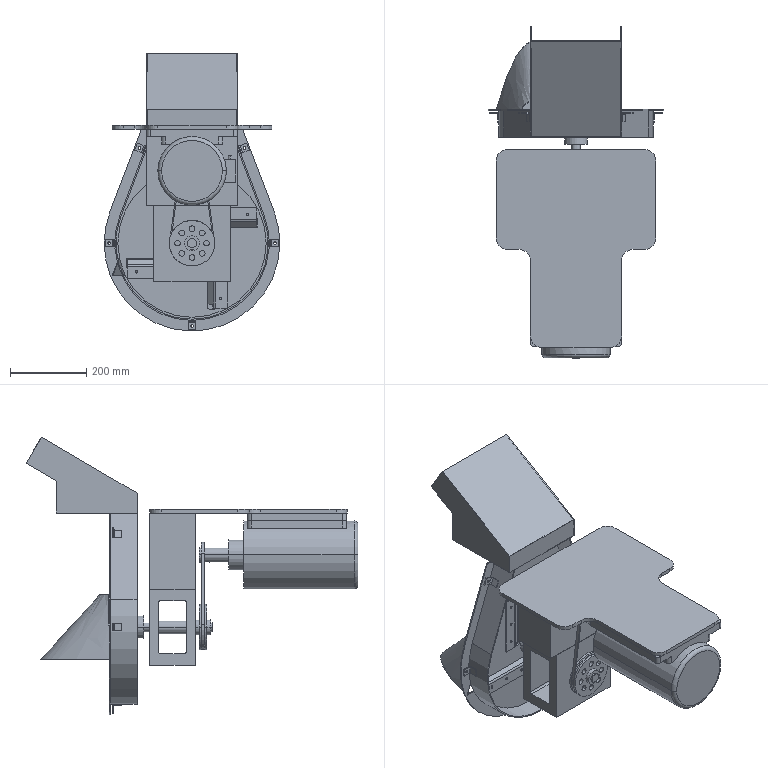Part | SolidWorks | features AEMSimFeature 1 | 54 solids | 733 faces | box 462 x 872.289 x 730.81 mm | volume 20879120 mm3 | plane 276 | cylinder 261 | sphere 112 | cone 56 | torus 26 | spline 2 | commonest cylinder face diameters 7 x68 10 x42 15 x16 60 x14 16 x12 24 x10